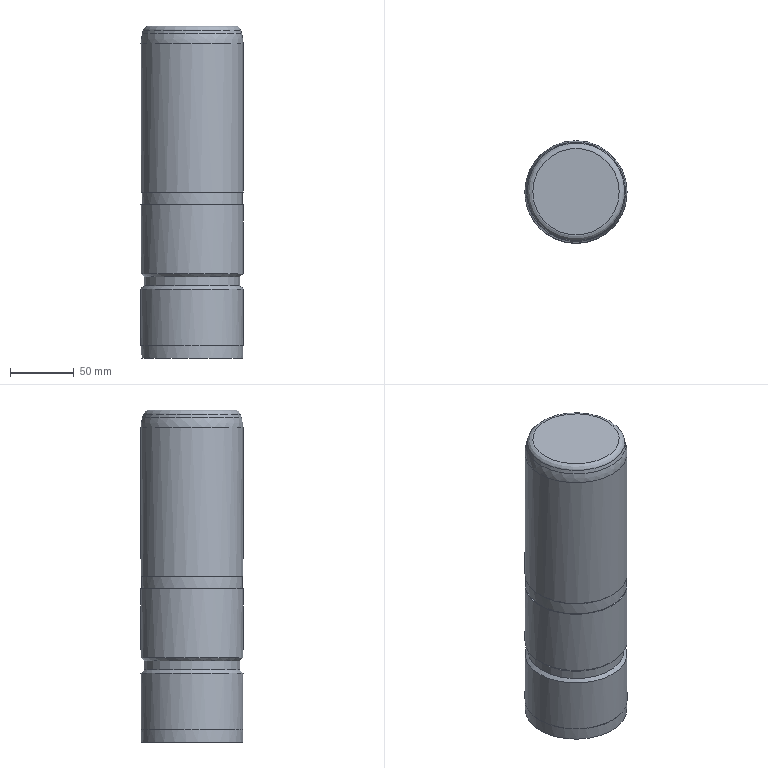Part | NX | features solid 2 | 1 solid | 16 faces | box 80 x 80 x 260 mm | volume 1295239 mm3 | cylinder 6 | plane 5 | cone 3 | torus 2 | commonest cylinder face diameters 80 x3 75 x1 79 x1 79.5 x1
STEP:
#1=CARTESIAN_POINT('',(-1297.5,-510.,-221.5));
#2=VERTEX_POINT('',#1);
#3=CARTESIAN_POINT('',(-1260.,-510.,-221.5));
#4=DIRECTION('',(0.,0.,1.));
#5=DIRECTION('',(-1.,0.,0.));
#6=AXIS2_PLACEMENT_3D('',#3,#4,#5);
#7=CIRCLE('',#6,37.5);
#8=EDGE_CURVE('',#2,#2,#7,.T.);
#9=ORIENTED_EDGE('',*,*,#8,.T.);
#10=EDGE_LOOP('',(#9));
#11=FACE_BOUND('',#10,.T.);
#12=CARTESIAN_POINT('',(-1220.,-510.,-219.));
#13=VERTEX_POINT('',#12);
#14=CARTESIAN_POINT('',(-1260.,-510.,-219.));
#15=DIRECTION('',(0.,0.,-1.));
#16=DIRECTION('',(1.,0.,0.));
#17=AXIS2_PLACEMENT_3D('',#14,#15,#16);
#18=CIRCLE('',#17,40.);
#19=EDGE_CURVE('',#13,#13,#18,.T.);
#20=ORIENTED_EDGE('',*,*,#19,.T.);
#21=EDGE_LOOP('',(#20));
#22=FACE_BOUND('',#21,.T.);
#23=CARTESIAN_POINT('',(-1260.,-510.,-221.5));
#24=DIRECTION('',(0.,0.,1.));
#25=DIRECTION('',(1.,0.,0.));
#26=AXIS2_PLACEMENT_3D('',#23,#24,#25);
#27=CONICAL_SURFACE('',#26,37.5,0.7854);
#28=ADVANCED_FACE('',(#11,#22),#27,.T.);
#29=ORIENTED_EDGE('',*,*,#8,.F.);
#30=EDGE_LOOP('',(#29));
#31=FACE_BOUND('',#30,.T.);
#32=CARTESIAN_POINT('',(-1297.5,-510.,-228.5));
#33=VERTEX_POINT('',#32);
#34=CARTESIAN_POINT('',(-1260.,-510.,-228.5));
#35=DIRECTION('',(0.,0.,1.));
#36=DIRECTION('',(-1.,0.,0.));
#37=AXIS2_PLACEMENT_3D('',#34,#35,#36);
#38=CIRCLE('',#37,37.5);
#39=EDGE_CURVE('',#33,#33,#38,.T.);
#40=ORIENTED_EDGE('',*,*,#39,.T.);
#41=EDGE_LOOP('',(#40));
#42=FACE_BOUND('',#41,.T.);
#43=CARTESIAN_POINT('',(-1260.,-510.,-228.5));
#44=DIRECTION('',(0.,0.,1.));
#45=DIRECTION('',(1.,0.,0.));
#46=AXIS2_PLACEMENT_3D('',#43,#44,#45);
#47=CYLINDRICAL_SURFACE('',#46,37.5);
#48=ADVANCED_FACE('',(#31,#42),#47,.T.);
#49=CARTESIAN_POINT('',(-1220.5,-510.,-165.));
#50=VERTEX_POINT('',#49);
#51=CARTESIAN_POINT('',(-1260.,-510.,-165.));
#52=DIRECTION('',(0.,0.,-1.));
#53=DIRECTION('',(1.,0.,0.));
#54=AXIS2_PLACEMENT_3D('',#51,#52,#53);
#55=CIRCLE('',#54,39.5);
#56=EDGE_CURVE('',#50,#50,#55,.T.);
#57=ORIENTED_EDGE('',*,*,#56,.T.);
#58=EDGE_LOOP('',(#57));
#59=FACE_BOUND('',#58,.T.);
#60=CARTESIAN_POINT('',(-1300.,-510.,-165.));
#61=VERTEX_POINT('',#60);
#62=CARTESIAN_POINT('',(-1260.,-510.,-165.));
#63=DIRECTION('',(0.,0.,1.));
#64=DIRECTION('',(-1.,0.,0.));
#65=AXIS2_PLACEMENT_3D('',#62,#63,#64);
#66=CIRCLE('',#65,40.);
#67=EDGE_CURVE('',#61,#61,#66,.T.);
#68=ORIENTED_EDGE('',*,*,#67,.T.);
#69=EDGE_LOOP('',(#68));
#70=FACE_BOUND('',#69,.T.);
#71=CARTESIAN_POINT('',(-1260.,-510.,-165.));
#72=DIRECTION('',(0.,0.,1.));
#73=DIRECTION('',(1.,0.,0.));
#74=AXIS2_PLACEMENT_3D('',#71,#72,#73);
#75=PLANE('',#74);
#76=ADVANCED_FACE('',(#59,#70),#75,.T.);
#77=ORIENTED_EDGE('',*,*,#67,.F.);
#78=EDGE_LOOP('',(#77));
#79=FACE_BOUND('',#78,.T.);
#80=ORIENTED_EDGE('',*,*,#19,.F.);
#81=EDGE_LOOP('',(#80));
#82=FACE_BOUND('',#81,.T.);
#83=CARTESIAN_POINT('',(-1260.,-510.,-219.));
#84=DIRECTION('',(0.,0.,1.));
#85=DIRECTION('',(1.,0.,0.));
#86=AXIS2_PLACEMENT_3D('',#83,#84,#85);
#87=CYLINDRICAL_SURFACE('',#86,40.);
#88=ADVANCED_FACE('',(#79,#82),#87,.T.);
#89=CARTESIAN_POINT('',(-1299.5,-510.,-155.));
#90=VERTEX_POINT('',#89);
#91=CARTESIAN_POINT('',(-1260.,-510.,-155.));
#92=DIRECTION('',(0.,0.,1.));
#93=DIRECTION('',(-1.,0.,0.));
#94=AXIS2_PLACEMENT_3D('',#91,#92,#93);
#95=CIRCLE('',#94,39.5);
#96=EDGE_CURVE('',#90,#90,#95,.T.);
#97=ORIENTED_EDGE('',*,*,#96,.T.);
#98=EDGE_LOOP('',(#97));
#99=FACE_BOUND('',#98,.T.);
#100=CARTESIAN_POINT('',(-1220.,-510.,-155.));
#101=VERTEX_POINT('',#100);
#102=CARTESIAN_POINT('',(-1260.,-510.,-155.));
#103=DIRECTION('',(0.,0.,-1.));
#104=DIRECTION('',(1.,0.,0.));
#105=AXIS2_PLACEMENT_3D('',#102,#103,#104);
#106=CIRCLE('',#105,40.);
#107=EDGE_CURVE('',#101,#101,#106,.T.);
#108=ORIENTED_EDGE('',*,*,#107,.T.);
#109=EDGE_LOOP('',(#108));
#110=FACE_BOUND('',#109,.T.);
#111=CARTESIAN_POINT('',(-1260.,-510.,-155.));
#112=DIRECTION('',(0.,0.,-1.));
#113=DIRECTION('',(-1.,0.,0.));
#114=AXIS2_PLACEMENT_3D('',#111,#112,#113);
#115=PLANE('',#114);
#116=ADVANCED_FACE('',(#99,#110),#115,.T.);
#117=CARTESIAN_POINT('',(-1300.,-510.,-38.95));
#118=VERTEX_POINT('',#117);
#119=CARTESIAN_POINT('',(-1260.,-510.,-38.95));
#120=DIRECTION('',(0.,0.,1.));
#121=DIRECTION('',(-1.,0.,0.));
#122=AXIS2_PLACEMENT_3D('',#119,#120,#121);
#123=CIRCLE('',#122,40.);
#124=EDGE_CURVE('',#118,#118,#123,.T.);
#125=ORIENTED_EDGE('',*,*,#124,.F.);
#126=EDGE_LOOP('',(#125));
#127=FACE_BOUND('',#126,.T.);
#128=ORIENTED_EDGE('',*,*,#107,.F.);
#129=EDGE_LOOP('',(#128));
#130=FACE_BOUND('',#129,.T.);
#131=CARTESIAN_POINT('',(-1260.,-510.,-155.));
#132=DIRECTION('',(0.,0.,1.));
#133=DIRECTION('',(1.,0.,0.));
#134=AXIS2_PLACEMENT_3D('',#131,#132,#133);
#135=CYLINDRICAL_SURFACE('',#134,40.);
#136=ADVANCED_FACE('',(#127,#130),#135,.T.);
#137=ORIENTED_EDGE('',*,*,#96,.F.);
#138=EDGE_LOOP('',(#137));
#139=FACE_BOUND('',#138,.T.);
#140=ORIENTED_EDGE('',*,*,#56,.F.);
#141=EDGE_LOOP('',(#140));
#142=FACE_BOUND('',#141,.T.);
#143=CARTESIAN_POINT('',(-1260.,-510.,-165.));
#144=DIRECTION('',(0.,0.,1.));
#145=DIRECTION('',(1.,0.,0.));
#146=AXIS2_PLACEMENT_3D('',#143,#144,#145);
#147=CYLINDRICAL_SURFACE('',#146,39.5);
#148=ADVANCED_FACE('',(#139,#142),#147,.T.);
#149=CARTESIAN_POINT('',(-1226.132,-510.,-25.));
#150=VERTEX_POINT('',#149);
#151=CARTESIAN_POINT('',(-1260.,-510.,-25.));
#152=DIRECTION('',(0.,0.,-1.));
#153=DIRECTION('',(1.,0.,0.));
#154=AXIS2_PLACEMENT_3D('',#151,#152,#153);
#155=CIRCLE('',#154,33.868);
#156=EDGE_CURVE('',#150,#150,#155,.T.);
#157=ORIENTED_EDGE('',*,*,#156,.F.);
#158=EDGE_LOOP('',(#157));
#159=FACE_BOUND('',#158,.T.);
#160=CARTESIAN_POINT('',(-1260.,-510.,-25.));
#161=DIRECTION('',(0.,0.,1.));
#162=DIRECTION('',(1.,0.,0.));
#163=AXIS2_PLACEMENT_3D('',#160,#161,#162);
#164=PLANE('',#163);
#165=ADVANCED_FACE('',(#159),#164,.T.);
#166=CARTESIAN_POINT('',(-1221.786,-510.,-28.335));
#167=VERTEX_POINT('',#166);
#168=CARTESIAN_POINT('',(-1260.,-510.,-28.335));
#169=DIRECTION('',(0.,0.,-1.));
#170=DIRECTION('',(1.,0.,0.));
#171=AXIS2_PLACEMENT_3D('',#168,#169,#170);
#172=CIRCLE('',#171,38.214);
#173=EDGE_CURVE('',#167,#167,#172,.F.);
#174=ORIENTED_EDGE('',*,*,#173,.F.);
#175=EDGE_LOOP('',(#174));
#176=FACE_BOUND('',#175,.T.);
#177=CARTESIAN_POINT('',(-1221.022,-510.,-31.185));
#178=VERTEX_POINT('',#177);
#179=CARTESIAN_POINT('',(-1260.,-510.,-31.185));
#180=DIRECTION('',(0.,0.,-1.));
#181=DIRECTION('',(1.,0.,0.));
#182=AXIS2_PLACEMENT_3D('',#179,#180,#181);
#183=CIRCLE('',#182,38.978);
#184=EDGE_CURVE('',#178,#178,#183,.T.);
#185=ORIENTED_EDGE('',*,*,#184,.F.);
#186=EDGE_LOOP('',(#185));
#187=FACE_BOUND('',#186,.T.);
#188=CARTESIAN_POINT('',(-1260.,-510.,-25.));
#189=DIRECTION('',(0.,0.,-1.));
#190=DIRECTION('',(-1.,0.,0.));
#191=AXIS2_PLACEMENT_3D('',#188,#189,#190);
#192=CONICAL_SURFACE('',#191,37.321,0.2618);
#193=ADVANCED_FACE('',(#176,#187),#192,.T.);
#194=CARTESIAN_POINT('',(-1299.75,-510.,-275.));
#195=VERTEX_POINT('',#194);
#196=CARTESIAN_POINT('',(-1260.,-510.,-275.));
#197=DIRECTION('',(0.,0.,1.));
#198=DIRECTION('',(-1.,0.,0.));
#199=AXIS2_PLACEMENT_3D('',#196,#197,#198);
#200=CIRCLE('',#199,39.75);
#201=EDGE_CURVE('',#195,#195,#200,.T.);
#202=ORIENTED_EDGE('',*,*,#201,.T.);
#203=EDGE_LOOP('',(#202));
#204=FACE_BOUND('',#203,.T.);
#205=CARTESIAN_POINT('',(-1220.,-510.,-275.));
#206=VERTEX_POINT('',#205);
#207=CARTESIAN_POINT('',(-1260.,-510.,-275.));
#208=DIRECTION('',(0.,0.,-1.));
#209=DIRECTION('',(1.,0.,0.));
#210=AXIS2_PLACEMENT_3D('',#207,#208,#209);
#211=CIRCLE('',#210,40.);
#212=EDGE_CURVE('',#206,#206,#211,.T.);
#213=ORIENTED_EDGE('',*,*,#212,.T.);
#214=EDGE_LOOP('',(#213));
#215=FACE_BOUND('',#214,.T.);
#216=CARTESIAN_POINT('',(-1260.,-510.,-275.));
#217=DIRECTION('',(0.,0.,-1.));
#218=DIRECTION('',(-1.,0.,0.));
#219=AXIS2_PLACEMENT_3D('',#216,#217,#218);
#220=PLANE('',#219);
#221=ADVANCED_FACE('',(#204,#215),#220,.T.);
#222=CARTESIAN_POINT('',(-1220.,-510.,-231.));
#223=VERTEX_POINT('',#222);
#224=CARTESIAN_POINT('',(-1260.,-510.,-231.));
#225=DIRECTION('',(0.,0.,-1.));
#226=DIRECTION('',(1.,0.,0.));
#227=AXIS2_PLACEMENT_3D('',#224,#225,#226);
#228=CIRCLE('',#227,40.);
#229=EDGE_CURVE('',#223,#223,#228,.T.);
#230=ORIENTED_EDGE('',*,*,#229,.T.);
#231=EDGE_LOOP('',(#230));
#232=FACE_BOUND('',#231,.T.);
#233=ORIENTED_EDGE('',*,*,#212,.F.);
#234=EDGE_LOOP('',(#233));
#235=FACE_BOUND('',#234,.T.);
#236=CARTESIAN_POINT('',(-1260.,-510.,-275.));
#237=DIRECTION('',(0.,0.,1.));
#238=DIRECTION('',(1.,0.,0.));
#239=AXIS2_PLACEMENT_3D('',#236,#237,#238);
#240=CYLINDRICAL_SURFACE('',#239,40.);
#241=ADVANCED_FACE('',(#232,#235),#240,.T.);
#242=CARTESIAN_POINT('',(-1220.25,-510.,-285.));
#243=VERTEX_POINT('',#242);
#244=CARTESIAN_POINT('',(-1260.,-510.,-285.));
#245=DIRECTION('',(0.,0.,-1.));
#246=DIRECTION('',(1.,0.,0.));
#247=AXIS2_PLACEMENT_3D('',#244,#245,#246);
#248=CIRCLE('',#247,39.75);
#249=EDGE_CURVE('',#243,#243,#248,.T.);
#250=ORIENTED_EDGE('',*,*,#249,.T.);
#251=EDGE_LOOP('',(#250));
#252=FACE_BOUND('',#251,.T.);
#253=CARTESIAN_POINT('',(-1260.,-510.,-285.));
#254=DIRECTION('',(0.,0.,-1.));
#255=DIRECTION('',(-1.,0.,0.));
#256=AXIS2_PLACEMENT_3D('',#253,#254,#255);
#257=PLANE('',#256);
#258=ADVANCED_FACE('',(#252),#257,.T.);
#259=ORIENTED_EDGE('',*,*,#201,.F.);
#260=EDGE_LOOP('',(#259));
#261=FACE_BOUND('',#260,.T.);
#262=ORIENTED_EDGE('',*,*,#249,.F.);
#263=EDGE_LOOP('',(#262));
#264=FACE_BOUND('',#263,.T.);
#265=CARTESIAN_POINT('',(-1260.,-510.,-285.));
#266=DIRECTION('',(0.,0.,1.));
#267=DIRECTION('',(1.,0.,0.));
#268=AXIS2_PLACEMENT_3D('',#265,#266,#267);
#269=CYLINDRICAL_SURFACE('',#268,39.75);
#270=ADVANCED_FACE('',(#261,#264),#269,.T.);
#271=ORIENTED_EDGE('',*,*,#229,.F.);
#272=EDGE_LOOP('',(#271));
#273=FACE_BOUND('',#272,.T.);
#274=ORIENTED_EDGE('',*,*,#39,.F.);
#275=EDGE_LOOP('',(#274));
#276=FACE_BOUND('',#275,.T.);
#277=CARTESIAN_POINT('',(-1260.,-510.,-228.5));
#278=DIRECTION('',(0.,0.,-1.));
#279=DIRECTION('',(-1.,0.,0.));
#280=AXIS2_PLACEMENT_3D('',#277,#278,#279);
#281=CONICAL_SURFACE('',#280,37.5,0.7854);
#282=ADVANCED_FACE('',(#273,#276),#281,.T.);
#283=ORIENTED_EDGE('',*,*,#124,.T.);
#284=EDGE_LOOP('',(#283));
#285=FACE_BOUND('',#284,.T.);
#286=ORIENTED_EDGE('',*,*,#184,.T.);
#287=EDGE_LOOP('',(#286));
#288=FACE_BOUND('',#287,.T.);
#289=CARTESIAN_POINT('',(-1260.,-510.,-38.95));
#290=DIRECTION('',(0.,0.,-1.));
#291=DIRECTION('',(-1.,0.,0.));
#292=AXIS2_PLACEMENT_3D('',#289,#290,#291);
#293=DEGENERATE_TOROIDAL_SURFACE('',#292,10.,30.,.T.);
#294=ADVANCED_FACE('',(#285,#288),#293,.T.);
#295=ORIENTED_EDGE('',*,*,#156,.T.);
#296=EDGE_LOOP('',(#295));
#297=FACE_BOUND('',#296,.T.);
#298=ORIENTED_EDGE('',*,*,#173,.T.);
#299=EDGE_LOOP('',(#298));
#300=FACE_BOUND('',#299,.T.);
#301=CARTESIAN_POINT('',(-1260.,-510.,-29.5));
#302=DIRECTION('',(0.,0.,1.));
#303=DIRECTION('',(1.,0.,0.));
#304=AXIS2_PLACEMENT_3D('',#301,#302,#303);
#305=TOROIDAL_SURFACE('',#304,33.868,4.5);
#306=ADVANCED_FACE('',(#297,#300),#305,.T.);
#307=CLOSED_SHELL('',(#28,#48,#76,#88,#116,#136,#148,#165,#193,#221,#241,#258,#270,#282,#294,#306));
#308=MANIFOLD_SOLID_BREP('',#307);
#309=(LENGTH_UNIT()NAMED_UNIT(*)SI_UNIT(.MILLI.,.METRE.));
#310=UNCERTAINTY_MEASURE_WITH_UNIT(LENGTH_MEASURE(0.00001),#309,'','');
#311=(NAMED_UNIT(*)PLANE_ANGLE_UNIT()SI_UNIT($,.RADIAN.));
#312=(NAMED_UNIT(*)SI_UNIT($,.STERADIAN.)SOLID_ANGLE_UNIT());
#313=(GEOMETRIC_REPRESENTATION_CONTEXT(3)GLOBAL_UNCERTAINTY_ASSIGNED_CONTEXT((#310))GLOBAL_UNIT_ASSIGNED_CONTEXT((#309,#311,#312))REPRESENTATION_CONTEXT('',''));
#314=ADVANCED_BREP_SHAPE_REPRESENTATION('',(#308),#313);